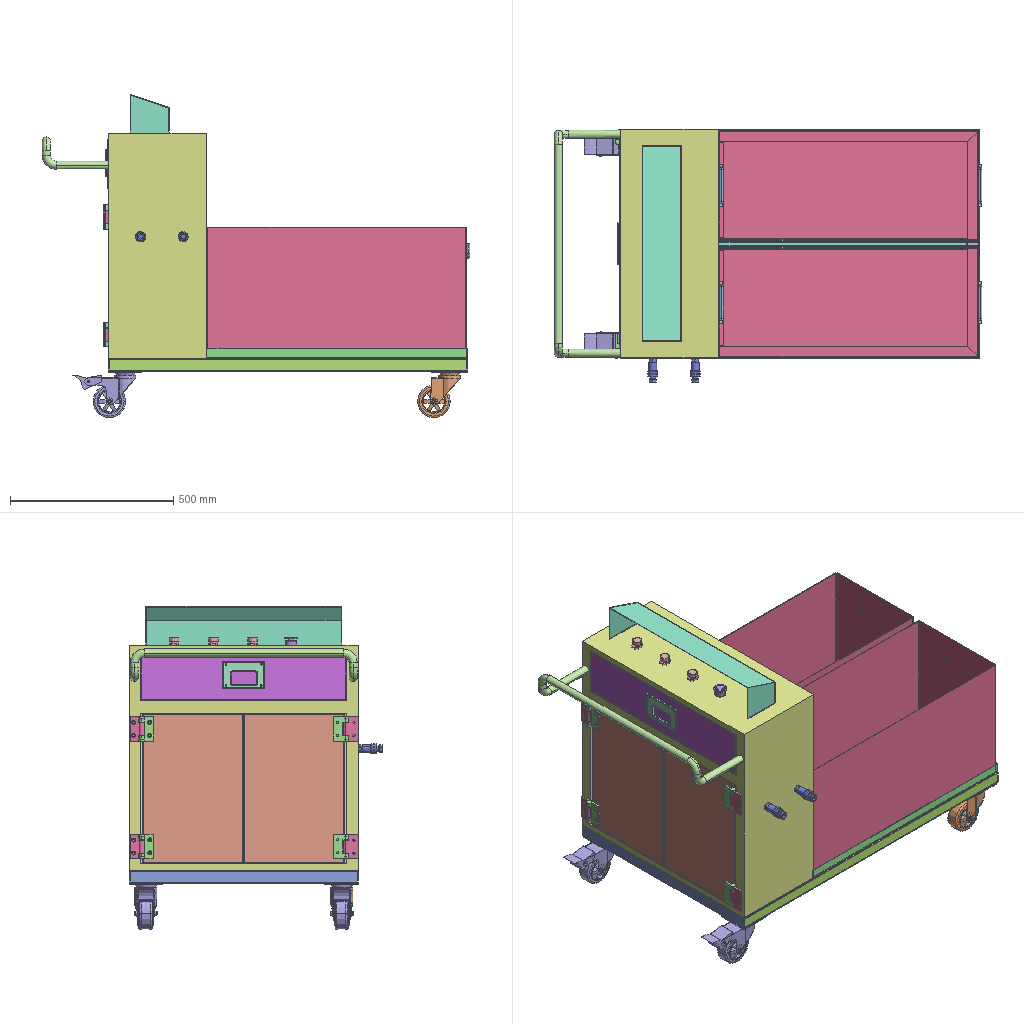Assembly | SolidWorks | 20 different items | 38 placed | box 1309 x 775 x 989 mm
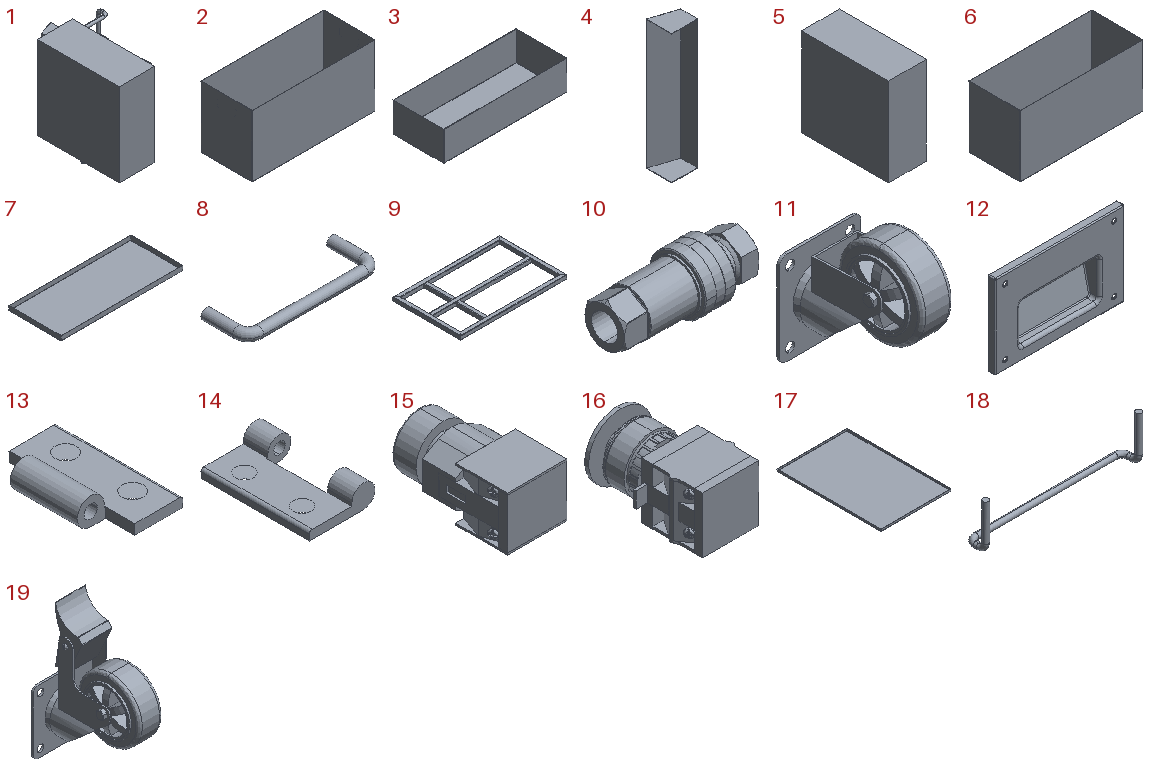Parts list (item | name | quantity | parent item | size | volume | features):
1 | (subassembly) | x1 | - | 502.5 x 808 x 775 mm | 40067990 mm3 | features ReferencePattern 10, LocalLPattern 3, AEMSimFeature 1, MirrorCompFeat 1
2 | (subassembly) | x2 | - | 805 x 335 x 400 mm | 2340531 mm3 | features AEMSimFeature 1
3 | - | x1 | in 1 | 630 x 260 x 150 mm | 844986 mm3 | features EdgeFlange 1, FlatPattern 1, SMBaseFlange 1, SheetMetal 1
4 | - | x1 | in 1 | 120 x 118 x 600 mm | 288678 mm3 | features Extrusion 1, ICE 1, Shell 1
5 | - | x1 | in 1 | 300 x 690 x 700 mm | 37296000 mm3 | features ICE 2, Extrusion 1
6 | - | x2 | in 2 | 795 x 335 x 400 mm | 2310463 mm3 | features EdgeFlange 1, FlatPattern 1, SMBaseFlange 1, SheetMetal 1
7 | - | x2 | - | 800 x 344 x 30 mm | 406893 mm3 | features EdgeFlange 1, FlatPattern 1, SMBaseFlange 1, SheetMetal 1
8 | - | x4 | in 2 | 130 x 45 x 10 mm | 15034 mm3 | features Sweep 1
9 | - | x1 | - | 1100 x 700 x 40 mm | 1480244 mm3 | features WeldMemberFeat 1, WeldmentFeature 1
10 | - | x2 | in 1 | 75 x 31.5 x 31.5 mm | 35275 mm3 | features BaseBody 1
11 | - | x2 | - | 96 x 142 x 153 mm | 354889 mm3 | features BaseBody 1
12 | - | x1 | in 1 | 128 x 18.75 x 83 mm | 17902 mm3 | features Cut 3, Fillet 3, Boss 1, Extrusion 1
13 | - | x4 | in 1 | - | - | features RefSurface 1
14 | - | x4 | in 1 | - | - | features RefSurface 1
15 | - | x3 | in 1 | 32.2 x 64 x 29 mm | 47816 mm3 | features BaseBody 4
16 | - | x1 | in 1 | 44.5 x 74 x 40 mm | 70679 mm3 | features BaseBody 5
17 | - | x2 | in 1 | 310 x 460 x 10 mm | 306822 mm3 | features EdgeFlange 1, FlatPattern 1, SMBaseFlange 1, SheetMetal 1
18 | - | x1 | in 1 | 695 x 99.162 x 202.5 mm | 562944 mm3 | features 3DProfileFeature 2, Sweep 1
19 | - | x2 | - | 102 x 142 x 213 mm | 452222 mm3 | features BaseBody 1
20 | Q11F-40T╱Q11F-25T Brass Ball Valve[DN40] | x1 | - | - | - | -
Mates (type | each side: item.copy, entity, surface, feature):
In the top assembly
Coincident | 9.1 face plane Structural cold-formed square tube (GB/T 6728) 40X2(1) | 7.1 face plane Base-Flange1
Coincident | 9.1 face plane Structural cold-formed square tube (GB/T 6728) 40X2(1) | 7.1 face plane Edge-Flange1 | 2 times
Coincident | 7.1 face plane Base-Flange1 | 6.1 face plane Base-Flange1
DistanceDim | 7.1 face plane Edge-Flange1 | 6.1 face plane Edge-Flange1
DistanceDim | 6.1 face plane Edge-Flange1 | 7.1 face plane Edge-Flange1
Coincident | 9.1 face plane Structural cold-formed square tube (GB/T 6728) 40X2(1) | 5.1 face plane Boss-Extrude1 | 3 times
Coincident | 9.1 face plane Structural cold-formed square tube (GB/T 6728) 40X2(1) | 19.1 face plane Input1 | 3 times
Coincident | 9.1 face plane Structural cold-formed square tube (GB/T 6728) 40X2(1) | 11.1 face plane Input1 | 3 times
In subassembly 2
Coincident | 6.2 plane | 8.1 plane
DistanceDim | 8.1 face plane Sweep1 | 6.2 face plane Edge-Flange1
Tangent | 6.2 face plane Edge-Flange1 | 8.1 face cylinder Sweep1
Coincident | 8.1 face plane Sweep1 | 8.2 face plane Sweep1
Coincident | 8.2 plane | 2.1 plane
Tangent | 6.2 face plane Edge-Flange1 | 8.2 face cylinder Sweep1
In subassembly 1
Coincident | 5.2 face plane Cut-Extrude1 | 3.1 face plane Base-Flange1
Coincident | 5.2 face plane Cut-Extrude1 | 3.1 face plane Edge-Flange1
Coincident | 3.1 face plane Edge-Flange1 | 12.1 face plane Extrude1
DistanceDim | 3.1 face plane Edge-Flange1 | 12.1 face plane Extrude1
Coincident | 3.1 plane | 12.1 plane
Concentric | 14.1 face cylinder Surface-Input1 | 13.1 face cylinder Surface-Input1
Coincident | 14.1 face plane Surface-Input1 | 13.1 face plane Surface-Input1
Coincident | 5.2 face plane Boss-Extrude1 | 13.1 face plane Surface-Input1 | 2 times
DistanceDim | 13.1 face plane Surface-Input1 | 5.2 face plane Cut-Extrude2
Coincident | 14.1 face plane Surface-Input1 | 17.1 face plane Base-Flange1
Coincident | 5.2 face plane Cut-Extrude2 | 17.1 face plane Edge-Flange1
DistanceDim | 17.1 face plane Edge-Flange1 | 14.1 face plane Surface-Input1
Parallel | 5.2 face plane Boss-Extrude1 | 17.2 face plane Base-Flange1
Coincident | 5.2 face plane Boss-Extrude1 | 10.1 face plane Input1
DistanceDim | 10.1 face plane Input1 | 5.2 face plane Boss-Extrude1
Coincident | 5.2 face plane Boss-Extrude1 | 18.1 face plane Sweep1
Coincident | 18.1 plane | 1.1 plane
Coincident | 5.2 face plane Boss-Extrude1 | 16.1 face plane Input4
DistanceDim | 15.1 face plane Input1 | 5.2 face plane Boss-Extrude1
Coincident | 5.2 face plane Boss-Extrude1 | 4.1 face plane Cut-Extrude1
Coincident | 4.1 plane | 1.1 plane